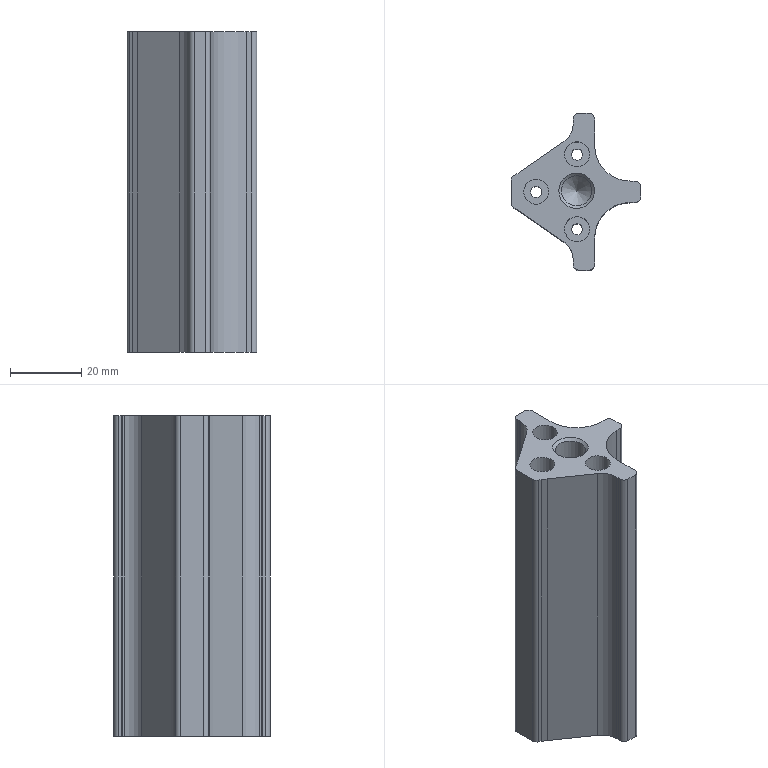Part | NX | features PU-16 2 | 1 solid | 46 faces | box 36.402 x 44 x 90 mm | volume 57632 mm3 | cylinder 23 | plane 19 | spline 2 | cone 2 | commonest cylinder face diameters 3 x8 3.101 x3 7 x3 10 x3 12 x2 20 x2